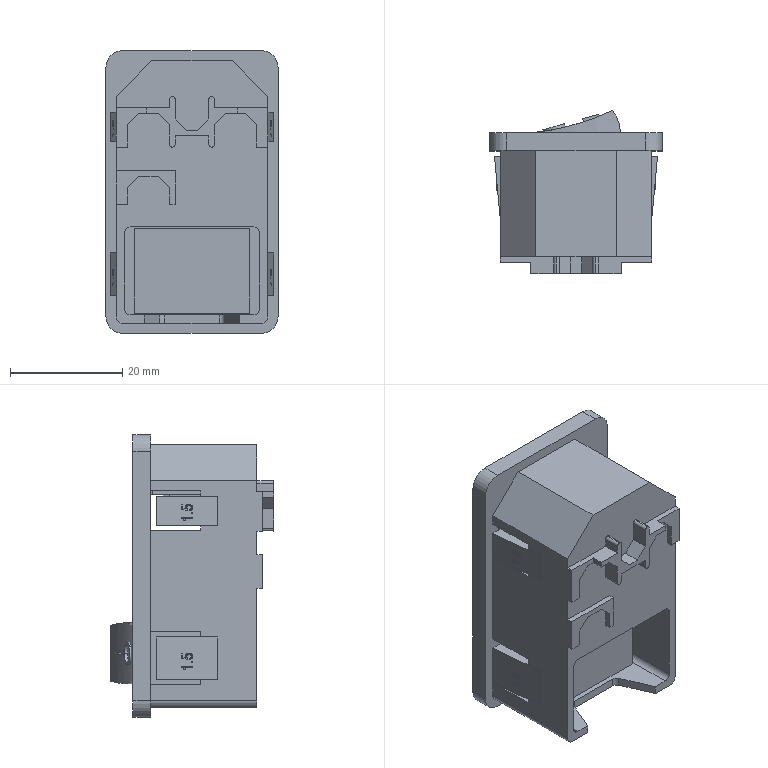Part | STEP file | 0004 | 1 solid | 582 faces | box 30.6 x 29.06 x 50.3 mm | volume 18939 mm3 | plane 424 | other 120 | cylinder 38 | commonest cylinder face diameters 1 x14 2 x6 6 x4 96.422 x3 2.4 x2 3 x2